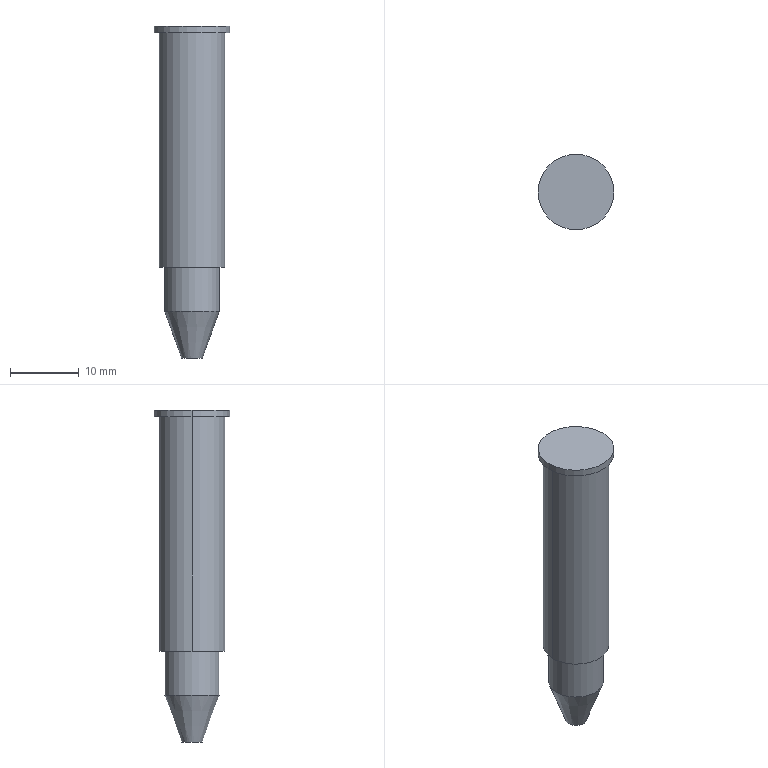Part | STEP file | 1_id262_x_t | 1 solid | 10 faces | box 11 x 11 x 48.205 mm | volume 3006 mm3 | cylinder 5 | plane 4 | cone 1 | commonest cylinder face diameters 9.525 x2 11 x2 7.94 x1
STEP:
#1=CARTESIAN_POINT('',(0.,0.,0.));
#2=DIRECTION('',(0.,0.,1.));
#3=DIRECTION('',(1.,0.,0.));
#4=AXIS2_PLACEMENT_3D('',#1,#2,#3);
#5=CARTESIAN_POINT('',(211.912,177.5,4.075));
#6=VERTEX_POINT('',#5);
#7=CARTESIAN_POINT('',(202.387,177.5,4.075));
#8=VERTEX_POINT('',#7);
#9=CARTESIAN_POINT('',(207.15,177.5,4.075));
#10=DIRECTION('',(0.,0.,1.));
#11=DIRECTION('',(-1.,0.,0.));
#12=AXIS2_PLACEMENT_3D('',#9,#10,#11);
#13=CIRCLE('',#12,4.763);
#14=CARTESIAN_POINT('',(274.812,177.5,4.075));
#15=DIRECTION('',(0.,0.,-1.));
#16=DIRECTION('',(-1.,0.,0.));
#17=AXIS2_PLACEMENT_3D('',#14,#15,#16);
#18=PLANE('',#17);
#19=CARTESIAN_POINT('',(72.425,0.));
#20=CARTESIAN_POINT('',(72.425,-8.249));
#21=CARTESIAN_POINT('',(65.281,-4.124));
#22=CARTESIAN_POINT('',(58.138,0.));
#23=CARTESIAN_POINT('',(65.281,4.124));
#24=CARTESIAN_POINT('',(72.425,8.249));
#25=CARTESIAN_POINT('',(72.425,0.));
#26=(BOUNDED_CURVE()B_SPLINE_CURVE(2,(#19,#20,#21,#22,#23,#24,#25),.UNSPECIFIED.,.T.,.F.)B_SPLINE_CURVE_WITH_KNOTS((1,2,2,2,2,1),(-2.094,0.,2.094,4.189,6.283,8.378),.UNSPECIFIED.)CURVE()GEOMETRIC_REPRESENTATION_ITEM()RATIONAL_B_SPLINE_CURVE((1.,0.5,1.,0.5,1.,0.5,1.))REPRESENTATION_ITEM(''));
#27=(GEOMETRIC_REPRESENTATION_CONTEXT(2)PARAMETRIC_REPRESENTATION_CONTEXT()REPRESENTATION_CONTEXT('',''));
#28=DEFINITIONAL_REPRESENTATION('',(#26),#27);
#29=PCURVE('',#18,#28);
#30=CARTESIAN_POINT('',(207.15,177.5,50.685));
#31=DIRECTION('',(0.,0.,-1.));
#32=DIRECTION('',(-1.,0.,0.));
#33=AXIS2_PLACEMENT_3D('',#30,#31,#32);
#34=CYLINDRICAL_SURFACE('',#33,4.763);
#35=CARTESIAN_POINT('',(6.283,46.61));
#36=DIRECTION('',(-1.,0.));
#37=VECTOR('',#36,1.);
#38=LINE('',#35,#37);
#39=(GEOMETRIC_REPRESENTATION_CONTEXT(2)PARAMETRIC_REPRESENTATION_CONTEXT()REPRESENTATION_CONTEXT('',''));
#40=DEFINITIONAL_REPRESENTATION('',(#38),#39);
#41=PCURVE('',#34,#40);
#42=SURFACE_CURVE('',#13,(#29,#41),.PCURVE_S1.);
#43=EDGE_CURVE('',#6,#8,#42,.T.);
#44=ORIENTED_EDGE('',*,*,#43,.F.);
#45=CARTESIAN_POINT('',(207.15,177.5,4.075));
#46=DIRECTION('',(0.,0.,1.));
#47=DIRECTION('',(-1.,0.,0.));
#48=AXIS2_PLACEMENT_3D('',#45,#46,#47);
#49=CIRCLE('',#48,4.763);
#50=CARTESIAN_POINT('',(72.425,0.));
#51=CARTESIAN_POINT('',(72.425,-8.249));
#52=CARTESIAN_POINT('',(65.281,-4.124));
#53=CARTESIAN_POINT('',(58.138,0.));
#54=CARTESIAN_POINT('',(65.281,4.124));
#55=CARTESIAN_POINT('',(72.425,8.249));
#56=CARTESIAN_POINT('',(72.425,0.));
#57=(BOUNDED_CURVE()B_SPLINE_CURVE(2,(#50,#51,#52,#53,#54,#55,#56),.UNSPECIFIED.,.T.,.F.)B_SPLINE_CURVE_WITH_KNOTS((1,2,2,2,2,1),(-2.094,0.,2.094,4.189,6.283,8.378),.UNSPECIFIED.)CURVE()GEOMETRIC_REPRESENTATION_ITEM()RATIONAL_B_SPLINE_CURVE((1.,0.5,1.,0.5,1.,0.5,1.))REPRESENTATION_ITEM(''));
#58=(GEOMETRIC_REPRESENTATION_CONTEXT(2)PARAMETRIC_REPRESENTATION_CONTEXT()REPRESENTATION_CONTEXT('',''));
#59=DEFINITIONAL_REPRESENTATION('',(#57),#58);
#60=PCURVE('',#18,#59);
#61=CARTESIAN_POINT('',(207.15,177.5,50.685));
#62=DIRECTION('',(0.,0.,-1.));
#63=DIRECTION('',(-1.,0.,0.));
#64=AXIS2_PLACEMENT_3D('',#61,#62,#63);
#65=CYLINDRICAL_SURFACE('',#64,4.763);
#66=CARTESIAN_POINT('',(6.283,46.61));
#67=DIRECTION('',(-1.,0.));
#68=VECTOR('',#67,1.);
#69=LINE('',#66,#68);
#70=(GEOMETRIC_REPRESENTATION_CONTEXT(2)PARAMETRIC_REPRESENTATION_CONTEXT()REPRESENTATION_CONTEXT('',''));
#71=DEFINITIONAL_REPRESENTATION('',(#69),#70);
#72=PCURVE('',#65,#71);
#73=SURFACE_CURVE('',#49,(#60,#72),.PCURVE_S1.);
#74=EDGE_CURVE('',#8,#6,#73,.T.);
#75=ORIENTED_EDGE('',*,*,#74,.F.);
#76=EDGE_LOOP('',(#44,#75));
#77=FACE_BOUND('',#76,.T.);
#78=CARTESIAN_POINT('',(203.18,177.5,4.075));
#79=VERTEX_POINT('',#78);
#80=CARTESIAN_POINT('',(207.15,177.5,4.075));
#81=DIRECTION('',(0.,0.,1.));
#82=DIRECTION('',(-1.,0.,0.));
#83=AXIS2_PLACEMENT_3D('',#80,#81,#82);
#84=CIRCLE('',#83,3.97);
#85=CARTESIAN_POINT('',(71.632,0.));
#86=CARTESIAN_POINT('',(71.632,-6.876));
#87=CARTESIAN_POINT('',(65.677,-3.438));
#88=CARTESIAN_POINT('',(59.722,0.));
#89=CARTESIAN_POINT('',(65.677,3.438));
#90=CARTESIAN_POINT('',(71.632,6.876));
#91=CARTESIAN_POINT('',(71.632,0.));
#92=(BOUNDED_CURVE()B_SPLINE_CURVE(2,(#85,#86,#87,#88,#89,#90,#91),.UNSPECIFIED.,.T.,.F.)B_SPLINE_CURVE_WITH_KNOTS((1,2,2,2,2,1),(-2.094,0.,2.094,4.189,6.283,8.378),.UNSPECIFIED.)CURVE()GEOMETRIC_REPRESENTATION_ITEM()RATIONAL_B_SPLINE_CURVE((1.,0.5,1.,0.5,1.,0.5,1.))REPRESENTATION_ITEM(''));
#93=(GEOMETRIC_REPRESENTATION_CONTEXT(2)PARAMETRIC_REPRESENTATION_CONTEXT()REPRESENTATION_CONTEXT('',''));
#94=DEFINITIONAL_REPRESENTATION('',(#92),#93);
#95=PCURVE('',#18,#94);
#96=CARTESIAN_POINT('',(207.15,177.5,50.685));
#97=DIRECTION('',(0.,0.,-1.));
#98=DIRECTION('',(-1.,0.,0.));
#99=AXIS2_PLACEMENT_3D('',#96,#97,#98);
#100=CYLINDRICAL_SURFACE('',#99,3.97);
#101=CARTESIAN_POINT('',(6.283,46.61));
#102=DIRECTION('',(-1.,0.));
#103=VECTOR('',#102,1.);
#104=LINE('',#101,#103);
#105=(GEOMETRIC_REPRESENTATION_CONTEXT(2)PARAMETRIC_REPRESENTATION_CONTEXT()REPRESENTATION_CONTEXT('',''));
#106=DEFINITIONAL_REPRESENTATION('',(#104),#105);
#107=PCURVE('',#100,#106);
#108=SURFACE_CURVE('',#84,(#95,#107),.PCURVE_S1.);
#109=EDGE_CURVE('',#79,#79,#108,.T.);
#110=ORIENTED_EDGE('',*,*,#109,.T.);
#111=EDGE_LOOP('',(#110));
#112=FACE_BOUND('',#111,.T.);
#113=ADVANCED_FACE('',(#77,#112),#18,.T.);
#114=CARTESIAN_POINT('',(211.912,177.5,38.075));
#115=VERTEX_POINT('',#114);
#116=CARTESIAN_POINT('',(211.912,177.5,38.075));
#117=DIRECTION('',(0.,0.,1.));
#118=VECTOR('',#117,1.);
#119=LINE('',#116,#118);
#120=CARTESIAN_POINT('',(3.142,12.61));
#121=DIRECTION('',(0.,-1.));
#122=VECTOR('',#121,1.);
#123=LINE('',#120,#122);
#124=(GEOMETRIC_REPRESENTATION_CONTEXT(2)PARAMETRIC_REPRESENTATION_CONTEXT()REPRESENTATION_CONTEXT('',''));
#125=DEFINITIONAL_REPRESENTATION('',(#123),#124);
#126=PCURVE('',#34,#125);
#127=CARTESIAN_POINT('',(3.142,12.61));
#128=DIRECTION('',(0.,-1.));
#129=VECTOR('',#128,1.);
#130=LINE('',#127,#129);
#131=(GEOMETRIC_REPRESENTATION_CONTEXT(2)PARAMETRIC_REPRESENTATION_CONTEXT()REPRESENTATION_CONTEXT('',''));
#132=DEFINITIONAL_REPRESENTATION('',(#130),#131);
#133=PCURVE('',#65,#132);
#134=SURFACE_CURVE('',#119,(#126,#133),.PCURVE_S1.);
#135=EDGE_CURVE('',#6,#115,#134,.T.);
#136=ORIENTED_EDGE('',*,*,#135,.F.);
#137=ORIENTED_EDGE('',*,*,#43,.T.);
#138=CARTESIAN_POINT('',(202.387,177.5,38.075));
#139=VERTEX_POINT('',#138);
#140=CARTESIAN_POINT('',(202.387,177.5,38.075));
#141=DIRECTION('',(0.,0.,-1.));
#142=VECTOR('',#141,1.);
#143=LINE('',#140,#142);
#144=CARTESIAN_POINT('',(0.,12.61));
#145=DIRECTION('',(0.,1.));
#146=VECTOR('',#145,1.);
#147=LINE('',#144,#146);
#148=(GEOMETRIC_REPRESENTATION_CONTEXT(2)PARAMETRIC_REPRESENTATION_CONTEXT()REPRESENTATION_CONTEXT('',''));
#149=DEFINITIONAL_REPRESENTATION('',(#147),#148);
#150=PCURVE('',#34,#149);
#151=CARTESIAN_POINT('',(6.283,12.61));
#152=DIRECTION('',(0.,1.));
#153=VECTOR('',#152,1.);
#154=LINE('',#151,#153);
#155=(GEOMETRIC_REPRESENTATION_CONTEXT(2)PARAMETRIC_REPRESENTATION_CONTEXT()REPRESENTATION_CONTEXT('',''));
#156=DEFINITIONAL_REPRESENTATION('',(#154),#155);
#157=PCURVE('',#65,#156);
#158=SURFACE_CURVE('',#143,(#150,#157),.PCURVE_S1.);
#159=EDGE_CURVE('',#139,#8,#158,.T.);
#160=ORIENTED_EDGE('',*,*,#159,.F.);
#161=CARTESIAN_POINT('',(207.15,177.5,38.075));
#162=DIRECTION('',(0.,0.,1.));
#163=DIRECTION('',(1.,0.,0.));
#164=AXIS2_PLACEMENT_3D('',#161,#162,#163);
#165=CIRCLE('',#164,4.763);
#166=CARTESIAN_POINT('',(3.142,12.61));
#167=DIRECTION('',(-1.,0.));
#168=VECTOR('',#167,1.);
#169=LINE('',#166,#168);
#170=(GEOMETRIC_REPRESENTATION_CONTEXT(2)PARAMETRIC_REPRESENTATION_CONTEXT()REPRESENTATION_CONTEXT('',''));
#171=DEFINITIONAL_REPRESENTATION('',(#169),#170);
#172=PCURVE('',#34,#171);
#173=CARTESIAN_POINT('',(207.15,177.5,38.075));
#174=DIRECTION('',(0.,0.,-1.));
#175=DIRECTION('',(-1.,0.,0.));
#176=AXIS2_PLACEMENT_3D('',#173,#174,#175);
#177=PLANE('',#176);
#178=CARTESIAN_POINT('',(-4.763,0.));
#179=CARTESIAN_POINT('',(-4.763,8.249));
#180=CARTESIAN_POINT('',(2.381,4.124));
#181=CARTESIAN_POINT('',(9.525,0.));
#182=CARTESIAN_POINT('',(2.381,-4.124));
#183=CARTESIAN_POINT('',(-4.763,-8.249));
#184=CARTESIAN_POINT('',(-4.763,0.));
#185=(BOUNDED_CURVE()B_SPLINE_CURVE(2,(#178,#179,#180,#181,#182,#183,#184),.UNSPECIFIED.,.T.,.F.)B_SPLINE_CURVE_WITH_KNOTS((1,2,2,2,2,1),(-2.094,0.,2.094,4.189,6.283,8.378),.UNSPECIFIED.)CURVE()GEOMETRIC_REPRESENTATION_ITEM()RATIONAL_B_SPLINE_CURVE((1.,0.5,1.,0.5,1.,0.5,1.))REPRESENTATION_ITEM(''));
#186=(GEOMETRIC_REPRESENTATION_CONTEXT(2)PARAMETRIC_REPRESENTATION_CONTEXT()REPRESENTATION_CONTEXT('',''));
#187=DEFINITIONAL_REPRESENTATION('',(#185),#186);
#188=PCURVE('',#177,#187);
#189=SURFACE_CURVE('',#165,(#172,#188),.PCURVE_S1.);
#190=EDGE_CURVE('',#115,#139,#189,.T.);
#191=ORIENTED_EDGE('',*,*,#190,.F.);
#192=EDGE_LOOP('',(#136,#137,#160,#191));
#193=FACE_BOUND('',#192,.T.);
#194=ADVANCED_FACE('',(#193),#34,.T.);
#195=ORIENTED_EDGE('',*,*,#159,.T.);
#196=ORIENTED_EDGE('',*,*,#74,.T.);
#197=ORIENTED_EDGE('',*,*,#135,.T.);
#198=CARTESIAN_POINT('',(207.15,177.5,38.075));
#199=DIRECTION('',(0.,0.,1.));
#200=DIRECTION('',(-1.,0.,0.));
#201=AXIS2_PLACEMENT_3D('',#198,#199,#200);
#202=CIRCLE('',#201,4.763);
#203=CARTESIAN_POINT('',(6.283,12.61));
#204=DIRECTION('',(-1.,0.));
#205=VECTOR('',#204,1.);
#206=LINE('',#203,#205);
#207=(GEOMETRIC_REPRESENTATION_CONTEXT(2)PARAMETRIC_REPRESENTATION_CONTEXT()REPRESENTATION_CONTEXT('',''));
#208=DEFINITIONAL_REPRESENTATION('',(#206),#207);
#209=PCURVE('',#65,#208);
#210=CARTESIAN_POINT('',(4.763,0.));
#211=CARTESIAN_POINT('',(4.763,-8.249));
#212=CARTESIAN_POINT('',(-2.381,-4.124));
#213=CARTESIAN_POINT('',(-9.525,0.));
#214=CARTESIAN_POINT('',(-2.381,4.124));
#215=CARTESIAN_POINT('',(4.763,8.249));
#216=CARTESIAN_POINT('',(4.763,0.));
#217=(BOUNDED_CURVE()B_SPLINE_CURVE(2,(#210,#211,#212,#213,#214,#215,#216),.UNSPECIFIED.,.T.,.F.)B_SPLINE_CURVE_WITH_KNOTS((1,2,2,2,2,1),(-2.094,0.,2.094,4.189,6.283,8.378),.UNSPECIFIED.)CURVE()GEOMETRIC_REPRESENTATION_ITEM()RATIONAL_B_SPLINE_CURVE((1.,0.5,1.,0.5,1.,0.5,1.))REPRESENTATION_ITEM(''));
#218=(GEOMETRIC_REPRESENTATION_CONTEXT(2)PARAMETRIC_REPRESENTATION_CONTEXT()REPRESENTATION_CONTEXT('',''));
#219=DEFINITIONAL_REPRESENTATION('',(#217),#218);
#220=PCURVE('',#177,#219);
#221=SURFACE_CURVE('',#202,(#209,#220),.PCURVE_S1.);
#222=EDGE_CURVE('',#139,#115,#221,.T.);
#223=ORIENTED_EDGE('',*,*,#222,.F.);
#224=EDGE_LOOP('',(#195,#196,#197,#223));
#225=FACE_BOUND('',#224,.T.);
#226=ADVANCED_FACE('',(#225),#65,.T.);
#227=CARTESIAN_POINT('',(201.65,177.5,39.075));
#228=VERTEX_POINT('',#227);
#229=CARTESIAN_POINT('',(212.65,177.5,39.075));
#230=VERTEX_POINT('',#229);
#231=CARTESIAN_POINT('',(207.15,177.5,39.075));
#232=DIRECTION('',(0.,0.,1.));
#233=DIRECTION('',(-1.,0.,0.));
#234=AXIS2_PLACEMENT_3D('',#231,#232,#233);
#235=CIRCLE('',#234,5.5);
#236=CARTESIAN_POINT('',(207.15,177.5,43.075));
#237=DIRECTION('',(0.,0.,-1.));
#238=DIRECTION('',(-1.,0.,0.));
#239=AXIS2_PLACEMENT_3D('',#236,#237,#238);
#240=CYLINDRICAL_SURFACE('',#239,5.5);
#241=CARTESIAN_POINT('',(6.283,4.));
#242=DIRECTION('',(-1.,0.));
#243=VECTOR('',#242,1.);
#244=LINE('',#241,#243);
#245=(GEOMETRIC_REPRESENTATION_CONTEXT(2)PARAMETRIC_REPRESENTATION_CONTEXT()REPRESENTATION_CONTEXT('',''));
#246=DEFINITIONAL_REPRESENTATION('',(#244),#245);
#247=PCURVE('',#240,#246);
#248=CARTESIAN_POINT('',(274.812,177.5,39.075));
#249=DIRECTION('',(0.,0.,-1.));
#250=DIRECTION('',(-1.,0.,0.));
#251=AXIS2_PLACEMENT_3D('',#248,#249,#250);
#252=PLANE('',#251);
#253=CARTESIAN_POINT('',(73.162,0.));
#254=CARTESIAN_POINT('',(73.162,-9.526));
#255=CARTESIAN_POINT('',(64.912,-4.763));
#256=CARTESIAN_POINT('',(56.663,0.));
#257=CARTESIAN_POINT('',(64.912,4.763));
#258=CARTESIAN_POINT('',(73.162,9.526));
#259=CARTESIAN_POINT('',(73.162,0.));
#260=(BOUNDED_CURVE()B_SPLINE_CURVE(2,(#253,#254,#255,#256,#257,#258,#259),.UNSPECIFIED.,.T.,.F.)B_SPLINE_CURVE_WITH_KNOTS((1,2,2,2,2,1),(-2.094,0.,2.094,4.189,6.283,8.378),.UNSPECIFIED.)CURVE()GEOMETRIC_REPRESENTATION_ITEM()RATIONAL_B_SPLINE_CURVE((1.,0.5,1.,0.5,1.,0.5,1.))REPRESENTATION_ITEM(''));
#261=(GEOMETRIC_REPRESENTATION_CONTEXT(2)PARAMETRIC_REPRESENTATION_CONTEXT()REPRESENTATION_CONTEXT('',''));
#262=DEFINITIONAL_REPRESENTATION('',(#260),#261);
#263=PCURVE('',#252,#262);
#264=SURFACE_CURVE('',#235,(#247,#263),.PCURVE_S1.);
#265=EDGE_CURVE('',#228,#230,#264,.T.);
#266=ORIENTED_EDGE('',*,*,#265,.F.);
#267=CARTESIAN_POINT('',(201.65,177.5,38.075));
#268=VERTEX_POINT('',#267);
#269=CARTESIAN_POINT('',(201.65,177.5,43.075));
#270=DIRECTION('',(0.,0.,1.));
#271=VECTOR('',#270,1.);
#272=LINE('',#269,#271);
#273=CARTESIAN_POINT('',(6.283,0.));
#274=DIRECTION('',(0.,-1.));
#275=VECTOR('',#274,1.);
#276=LINE('',#273,#275);
#277=(GEOMETRIC_REPRESENTATION_CONTEXT(2)PARAMETRIC_REPRESENTATION_CONTEXT()REPRESENTATION_CONTEXT('',''));
#278=DEFINITIONAL_REPRESENTATION('',(#276),#277);
#279=PCURVE('',#240,#278);
#280=CARTESIAN_POINT('',(207.15,177.5,43.075));
#281=DIRECTION('',(0.,0.,-1.));
#282=DIRECTION('',(-1.,0.,0.));
#283=AXIS2_PLACEMENT_3D('',#280,#281,#282);
#284=CYLINDRICAL_SURFACE('',#283,5.5);
#285=CARTESIAN_POINT('',(0.,0.));
#286=DIRECTION('',(0.,-1.));
#287=VECTOR('',#286,1.);
#288=LINE('',#285,#287);
#289=(GEOMETRIC_REPRESENTATION_CONTEXT(2)PARAMETRIC_REPRESENTATION_CONTEXT()REPRESENTATION_CONTEXT('',''));
#290=DEFINITIONAL_REPRESENTATION('',(#288),#289);
#291=PCURVE('',#284,#290);
#292=SURFACE_CURVE('',#272,(#279,#291),.PCURVE_S1.);
#293=EDGE_CURVE('',#268,#228,#292,.T.);
#294=ORIENTED_EDGE('',*,*,#293,.F.);
#295=CARTESIAN_POINT('',(212.65,177.5,38.075));
#296=VERTEX_POINT('',#295);
#297=CARTESIAN_POINT('',(207.15,177.5,38.075));
#298=DIRECTION('',(0.,0.,-1.));
#299=DIRECTION('',(1.,0.,0.));
#300=AXIS2_PLACEMENT_3D('',#297,#298,#299);
#301=CIRCLE('',#300,5.5);
#302=CARTESIAN_POINT('',(3.142,5.));
#303=DIRECTION('',(1.,0.));
#304=VECTOR('',#303,1.);
#305=LINE('',#302,#304);
#306=(GEOMETRIC_REPRESENTATION_CONTEXT(2)PARAMETRIC_REPRESENTATION_CONTEXT()REPRESENTATION_CONTEXT('',''));
#307=DEFINITIONAL_REPRESENTATION('',(#305),#306);
#308=PCURVE('',#240,#307);
#309=CARTESIAN_POINT('',(0.,0.));
#310=DIRECTION('',(-1.,0.));
#311=AXIS2_PLACEMENT_2D('',#309,#310);
#312=CIRCLE('',#311,5.5);
#313=(GEOMETRIC_REPRESENTATION_CONTEXT(2)PARAMETRIC_REPRESENTATION_CONTEXT()REPRESENTATION_CONTEXT('',''));
#314=DEFINITIONAL_REPRESENTATION('',(#312),#313);
#315=PCURVE('',#177,#314);
#316=SURFACE_CURVE('',#301,(#308,#315),.PCURVE_S1.);
#317=EDGE_CURVE('',#296,#268,#316,.T.);
#318=ORIENTED_EDGE('',*,*,#317,.F.);
#319=CARTESIAN_POINT('',(212.65,177.5,43.075));
#320=DIRECTION('',(0.,0.,-1.));
#321=VECTOR('',#320,1.);
#322=LINE('',#319,#321);
#323=CARTESIAN_POINT('',(3.142,0.));
#324=DIRECTION('',(0.,1.));
#325=VECTOR('',#324,1.);
#326=LINE('',#323,#325);
#327=(GEOMETRIC_REPRESENTATION_CONTEXT(2)PARAMETRIC_REPRESENTATION_CONTEXT()REPRESENTATION_CONTEXT('',''));
#328=DEFINITIONAL_REPRESENTATION('',(#326),#327);
#329=PCURVE('',#240,#328);
#330=CARTESIAN_POINT('',(3.142,0.));
#331=DIRECTION('',(0.,1.));
#332=VECTOR('',#331,1.);
#333=LINE('',#330,#332);
#334=(GEOMETRIC_REPRESENTATION_CONTEXT(2)PARAMETRIC_REPRESENTATION_CONTEXT()REPRESENTATION_CONTEXT('',''));
#335=DEFINITIONAL_REPRESENTATION('',(#333),#334);
#336=PCURVE('',#284,#335);
#337=SURFACE_CURVE('',#322,(#329,#336),.PCURVE_S1.);
#338=EDGE_CURVE('',#230,#296,#337,.T.);
#339=ORIENTED_EDGE('',*,*,#338,.F.);
#340=EDGE_LOOP('',(#266,#294,#318,#339));
#341=FACE_BOUND('',#340,.T.);
#342=ADVANCED_FACE('',(#341),#240,.T.);
#343=CARTESIAN_POINT('',(207.15,177.5,38.075));
#344=DIRECTION('',(0.,0.,-1.));
#345=DIRECTION('',(-1.,0.,0.));
#346=AXIS2_PLACEMENT_3D('',#343,#344,#345);
#347=CIRCLE('',#346,5.5);
#348=CARTESIAN_POINT('',(0.,0.));
#349=DIRECTION('',(1.,0.));
#350=AXIS2_PLACEMENT_2D('',#348,#349);
#351=CIRCLE('',#350,5.5);
#352=(GEOMETRIC_REPRESENTATION_CONTEXT(2)PARAMETRIC_REPRESENTATION_CONTEXT()REPRESENTATION_CONTEXT('',''));
#353=DEFINITIONAL_REPRESENTATION('',(#351),#352);
#354=PCURVE('',#177,#353);
#355=CARTESIAN_POINT('',(0.,5.));
#356=DIRECTION('',(1.,0.));
#357=VECTOR('',#356,1.);
#358=LINE('',#355,#357);
#359=(GEOMETRIC_REPRESENTATION_CONTEXT(2)PARAMETRIC_REPRESENTATION_CONTEXT()REPRESENTATION_CONTEXT('',''));
#360=DEFINITIONAL_REPRESENTATION('',(#358),#359);
#361=PCURVE('',#284,#360);
#362=SURFACE_CURVE('',#347,(#354,#361),.PCURVE_S1.);
#363=EDGE_CURVE('',#268,#296,#362,.T.);
#364=ORIENTED_EDGE('',*,*,#363,.T.);
#365=ORIENTED_EDGE('',*,*,#317,.T.);
#366=EDGE_LOOP('',(#364,#365));
#367=FACE_BOUND('',#366,.T.);
#368=ORIENTED_EDGE('',*,*,#222,.T.);
#369=ORIENTED_EDGE('',*,*,#190,.T.);
#370=EDGE_LOOP('',(#368,#369));
#371=FACE_BOUND('',#370,.T.);
#372=ADVANCED_FACE('',(#367,#371),#177,.T.);
#373=CARTESIAN_POINT('',(207.15,177.5,39.075));
#374=DIRECTION('',(0.,0.,1.));
#375=DIRECTION('',(-1.,0.,0.));
#376=AXIS2_PLACEMENT_3D('',#373,#374,#375);
#377=CIRCLE('',#376,5.5);
#378=CARTESIAN_POINT('',(6.283,4.));
#379=DIRECTION('',(-1.,0.));
#380=VECTOR('',#379,1.);
#381=LINE('',#378,#380);
#382=(GEOMETRIC_REPRESENTATION_CONTEXT(2)PARAMETRIC_REPRESENTATION_CONTEXT()REPRESENTATION_CONTEXT('',''));
#383=DEFINITIONAL_REPRESENTATION('',(#381),#382);
#384=PCURVE('',#284,#383);
#385=CARTESIAN_POINT('',(73.162,0.));
#386=CARTESIAN_POINT('',(73.162,-9.526));
#387=CARTESIAN_POINT('',(64.912,-4.763));
#388=CARTESIAN_POINT('',(56.663,0.));
#389=CARTESIAN_POINT('',(64.912,4.763));
#390=CARTESIAN_POINT('',(73.162,9.526));
#391=CARTESIAN_POINT('',(73.162,0.));
#392=(BOUNDED_CURVE()B_SPLINE_CURVE(2,(#385,#386,#387,#388,#389,#390,#391),.UNSPECIFIED.,.T.,.F.)B_SPLINE_CURVE_WITH_KNOTS((1,2,2,2,2,1),(-2.094,0.,2.094,4.189,6.283,8.378),.UNSPECIFIED.)CURVE()GEOMETRIC_REPRESENTATION_ITEM()RATIONAL_B_SPLINE_CURVE((1.,0.5,1.,0.5,1.,0.5,1.))REPRESENTATION_ITEM(''));
#393=(GEOMETRIC_REPRESENTATION_CONTEXT(2)PARAMETRIC_REPRESENTATION_CONTEXT()REPRESENTATION_CONTEXT('',''));
#394=DEFINITIONAL_REPRESENTATION('',(#392),#393);
#395=PCURVE('',#252,#394);
#396=SURFACE_CURVE('',#377,(#384,#395),.PCURVE_S1.);
#397=EDGE_CURVE('',#230,#228,#396,.T.);
#398=ORIENTED_EDGE('',*,*,#397,.F.);
#399=ORIENTED_EDGE('',*,*,#338,.T.);
#400=ORIENTED_EDGE('',*,*,#363,.F.);
#401=ORIENTED_EDGE('',*,*,#293,.T.);
#402=EDGE_LOOP('',(#398,#399,#400,#401));
#403=FACE_BOUND('',#402,.T.);
#404=ADVANCED_FACE('',(#403),#284,.T.);
#405=ORIENTED_EDGE('',*,*,#265,.T.);
#406=ORIENTED_EDGE('',*,*,#397,.T.);
#407=EDGE_LOOP('',(#405,#406));
#408=FACE_BOUND('',#407,.T.);
#409=ADVANCED_FACE('',(#408),#252,.F.);
#410=CARTESIAN_POINT('',(208.65,177.5,-9.13));
#411=VERTEX_POINT('',#410);
#412=CARTESIAN_POINT('',(207.15,177.5,-9.13));
#413=DIRECTION('',(0.,0.,-1.));
#414=DIRECTION('',(1.,0.,0.));
#415=AXIS2_PLACEMENT_3D('',#412,#413,#414);
#416=CIRCLE('',#415,1.5);
#417=CARTESIAN_POINT('',(207.15,177.5,-9.13));
#418=DIRECTION('',(0.,0.,-1.));
#419=DIRECTION('',(-1.,0.,0.));
#420=AXIS2_PLACEMENT_3D('',#417,#418,#419);
#421=PLANE('',#420);
#422=CARTESIAN_POINT('',(0.,0.));
#423=DIRECTION('',(-1.,0.));
#424=AXIS2_PLACEMENT_2D('',#422,#423);
#425=CIRCLE('',#424,1.5);
#426=(GEOMETRIC_REPRESENTATION_CONTEXT(2)PARAMETRIC_REPRESENTATION_CONTEXT()REPRESENTATION_CONTEXT('',''));
#427=DEFINITIONAL_REPRESENTATION('',(#425),#426);
#428=PCURVE('',#421,#427);
#429=CARTESIAN_POINT('',(207.15,177.5,-4.647));
#430=DIRECTION('',(0.,0.,1.));
#431=DIRECTION('',(1.,0.,0.));
#432=AXIS2_PLACEMENT_3D('',#429,#430,#431);
#433=CONICAL_SURFACE('',#432,3.131,0.3491);
#434=CARTESIAN_POINT('',(6.283,-4.482));
#435=DIRECTION('',(-1.,0.));
#436=VECTOR('',#435,1.);
#437=LINE('',#434,#436);
#438=(GEOMETRIC_REPRESENTATION_CONTEXT(2)PARAMETRIC_REPRESENTATION_CONTEXT()REPRESENTATION_CONTEXT('',''));
#439=DEFINITIONAL_REPRESENTATION('',(#437),#438);
#440=PCURVE('',#433,#439);
#441=SURFACE_CURVE('',#416,(#428,#440),.PCURVE_S1.);
#442=EDGE_CURVE('',#411,#411,#441,.T.);
#443=ORIENTED_EDGE('',*,*,#442,.T.);
#444=EDGE_LOOP('',(#443));
#445=FACE_BOUND('',#444,.T.);
#446=ADVANCED_FACE('',(#445),#421,.T.);
#447=CARTESIAN_POINT('',(211.12,177.5,-2.342));
#448=VERTEX_POINT('',#447);
#449=CARTESIAN_POINT('',(203.18,177.5,-2.342));
#450=VERTEX_POINT('',#449);
#451=CARTESIAN_POINT('',(207.15,177.5,-2.342));
#452=DIRECTION('',(0.,0.,-1.));
#453=DIRECTION('',(1.,0.,0.));
#454=AXIS2_PLACEMENT_3D('',#451,#452,#453);
#455=CIRCLE('',#454,3.97);
#456=CARTESIAN_POINT('',(6.283,2.305));
#457=DIRECTION('',(-1.,0.));
#458=VECTOR('',#457,1.);
#459=LINE('',#456,#458);
#460=(GEOMETRIC_REPRESENTATION_CONTEXT(2)PARAMETRIC_REPRESENTATION_CONTEXT()REPRESENTATION_CONTEXT('',''));
#461=DEFINITIONAL_REPRESENTATION('',(#459),#460);
#462=PCURVE('',#433,#461);
#463=CARTESIAN_POINT('',(3.142,53.027));
#464=DIRECTION('',(1.,0.));
#465=VECTOR('',#464,1.);
#466=LINE('',#463,#465);
#467=(GEOMETRIC_REPRESENTATION_CONTEXT(2)PARAMETRIC_REPRESENTATION_CONTEXT()REPRESENTATION_CONTEXT('',''));
#468=DEFINITIONAL_REPRESENTATION('',(#466),#467);
#469=PCURVE('',#100,#468);
#470=SURFACE_CURVE('',#455,(#462,#469),.PCURVE_S1.);
#471=EDGE_CURVE('',#448,#450,#470,.T.);
#472=ORIENTED_EDGE('',*,*,#471,.T.);
#473=CARTESIAN_POINT('',(207.15,177.5,-2.342));
#474=DIRECTION('',(0.,0.,-1.));
#475=DIRECTION('',(1.,0.,0.));
#476=AXIS2_PLACEMENT_3D('',#473,#474,#475);
#477=CIRCLE('',#476,3.97);
#478=CARTESIAN_POINT('',(6.283,2.305));
#479=DIRECTION('',(-1.,0.));
#480=VECTOR('',#479,1.);
#481=LINE('',#478,#480);
#482=(GEOMETRIC_REPRESENTATION_CONTEXT(2)PARAMETRIC_REPRESENTATION_CONTEXT()REPRESENTATION_CONTEXT('',''));
#483=DEFINITIONAL_REPRESENTATION('',(#481),#482);
#484=PCURVE('',#433,#483);
#485=CARTESIAN_POINT('',(-3.142,53.027));
#486=DIRECTION('',(1.,0.));
#487=VECTOR('',#486,1.);
#488=LINE('',#485,#487);
#489=(GEOMETRIC_REPRESENTATION_CONTEXT(2)PARAMETRIC_REPRESENTATION_CONTEXT()REPRESENTATION_CONTEXT('',''));
#490=DEFINITIONAL_REPRESENTATION('',(#488),#489);
#491=PCURVE('',#100,#490);
#492=SURFACE_CURVE('',#477,(#484,#491),.PCURVE_S1.);
#493=EDGE_CURVE('',#450,#448,#492,.T.);
#494=ORIENTED_EDGE('',*,*,#493,.T.);
#495=CARTESIAN_POINT('',(208.65,177.5,-9.13));
#496=CARTESIAN_POINT('',(211.12,177.5,-2.342));
#497=B_SPLINE_CURVE_WITH_KNOTS('',1,(#495,#496),.UNSPECIFIED.,.F.,.F.,(2,2),(-4.77,2.453),.PIECEWISE_BEZIER_KNOTS.);
#498=CARTESIAN_POINT('',(0.,0.));
#499=DIRECTION('',(0.,1.));
#500=VECTOR('',#499,1.);
#501=LINE('',#498,#500);
#502=(GEOMETRIC_REPRESENTATION_CONTEXT(2)PARAMETRIC_REPRESENTATION_CONTEXT()REPRESENTATION_CONTEXT('',''));
#503=DEFINITIONAL_REPRESENTATION('',(#501),#502);
#504=PCURVE('',#433,#503);
#505=CARTESIAN_POINT('',(6.283,0.));
#506=DIRECTION('',(0.,1.));
#507=VECTOR('',#506,1.);
#508=LINE('',#505,#507);
#509=(GEOMETRIC_REPRESENTATION_CONTEXT(2)PARAMETRIC_REPRESENTATION_CONTEXT()REPRESENTATION_CONTEXT('',''));
#510=DEFINITIONAL_REPRESENTATION('',(#508),#509);
#511=PCURVE('',#433,#510);
#512=SEAM_CURVE('',#497,(#504,#511),.PCURVE_S1.);
#513=EDGE_CURVE('',#411,#448,#512,.T.);
#514=ORIENTED_EDGE('',*,*,#513,.F.);
#515=ORIENTED_EDGE('',*,*,#442,.F.);
#516=ORIENTED_EDGE('',*,*,#513,.T.);
#517=EDGE_LOOP('',(#472,#494,#514,#515,#516));
#518=FACE_BOUND('',#517,.T.);
#519=ADVANCED_FACE('',(#518),#433,.T.);
#520=ORIENTED_EDGE('',*,*,#109,.F.);
#521=CARTESIAN_POINT('',(203.18,177.5,4.075));
#522=CARTESIAN_POINT('',(203.18,177.5,-2.342));
#523=B_SPLINE_CURVE_WITH_KNOTS('',1,(#521,#522),.UNSPECIFIED.,.F.,.F.,(2,2),(46.61,53.027),.PIECEWISE_BEZIER_KNOTS.);
#524=CARTESIAN_POINT('',(6.283,0.));
#525=DIRECTION('',(0.,1.));
#526=VECTOR('',#525,1.);
#527=LINE('',#524,#526);
#528=(GEOMETRIC_REPRESENTATION_CONTEXT(2)PARAMETRIC_REPRESENTATION_CONTEXT()REPRESENTATION_CONTEXT('',''));
#529=DEFINITIONAL_REPRESENTATION('',(#527),#528);
#530=PCURVE('',#100,#529);
#531=CARTESIAN_POINT('',(0.,0.));
#532=DIRECTION('',(0.,1.));
#533=VECTOR('',#532,1.);
#534=LINE('',#531,#533);
#535=(GEOMETRIC_REPRESENTATION_CONTEXT(2)PARAMETRIC_REPRESENTATION_CONTEXT()REPRESENTATION_CONTEXT('',''));
#536=DEFINITIONAL_REPRESENTATION('',(#534),#535);
#537=PCURVE('',#100,#536);
#538=SEAM_CURVE('',#523,(#530,#537),.PCURVE_S1.);
#539=EDGE_CURVE('',#79,#450,#538,.T.);
#540=ORIENTED_EDGE('',*,*,#539,.T.);
#541=ORIENTED_EDGE('',*,*,#471,.F.);
#542=ORIENTED_EDGE('',*,*,#493,.F.);
#543=ORIENTED_EDGE('',*,*,#539,.F.);
#544=EDGE_LOOP('',(#520,#540,#541,#542,#543));
#545=FACE_BOUND('',#544,.T.);
#546=ADVANCED_FACE('',(#545),#100,.T.);
#547=CLOSED_SHELL('',(#113,#194,#226,#342,#372,#404,#409,#446,#519,#546));
#548=MANIFOLD_SOLID_BREP('',#547);
#549=(LENGTH_UNIT()NAMED_UNIT(*)SI_UNIT(.MILLI.,.METRE.));
#550=UNCERTAINTY_MEASURE_WITH_UNIT(LENGTH_MEASURE(0.000002),#549,'','');
#551=(NAMED_UNIT(*)PLANE_ANGLE_UNIT()SI_UNIT($,.RADIAN.));
#552=(NAMED_UNIT(*)SI_UNIT($,.STERADIAN.)SOLID_ANGLE_UNIT());
#553=(GEOMETRIC_REPRESENTATION_CONTEXT(3)GLOBAL_UNCERTAINTY_ASSIGNED_CONTEXT((#550))GLOBAL_UNIT_ASSIGNED_CONTEXT((#549,#551,#552))REPRESENTATION_CONTEXT('',''));
#554=ADVANCED_BREP_SHAPE_REPRESENTATION('',(#4,#548),#553);